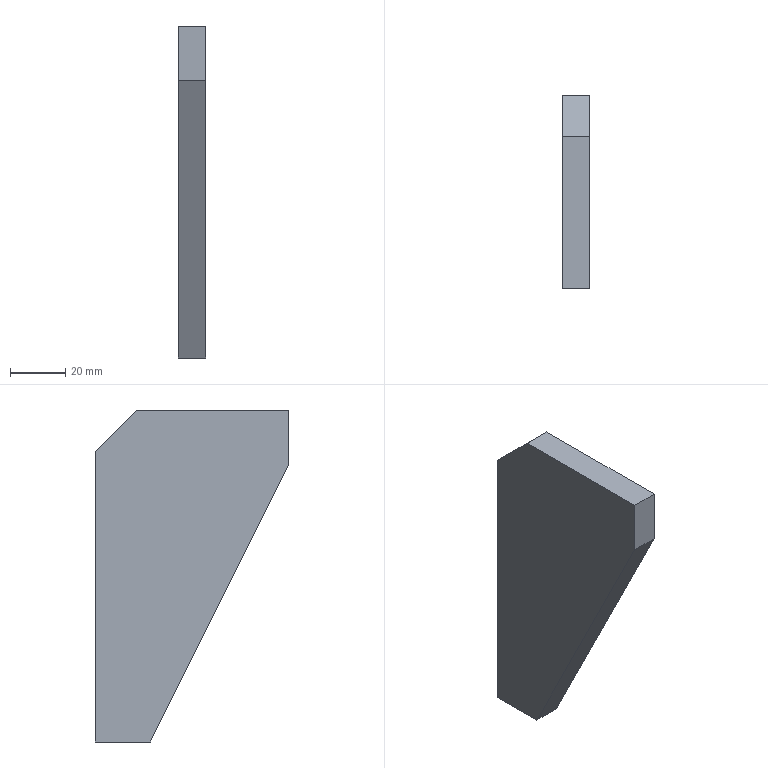Part | STEP file | VD-SYL0380DJ1006_1_4-2_VD-SYL03 | 1 solid | 8 faces | box 10 x 70 x 120 mm | volume 57804 mm3 | plane 8
STEP:
#1=CARTESIAN_POINT('',(0.,0.,-120.));
#2=VERTEX_POINT('',#1);
#3=CARTESIAN_POINT('',(0.,-20.,-120.));
#4=VERTEX_POINT('',#3);
#5=CARTESIAN_POINT('',(0.,0.,-120.));
#6=DIRECTION('',(0.,-1.,0.));
#7=VECTOR('',#6,1000.);
#8=LINE('',#5,#7);
#9=EDGE_CURVE('',#2,#4,#8,.T.);
#10=ORIENTED_EDGE('',*,*,#9,.T.);
#11=CARTESIAN_POINT('',(0.,-70.,-19.716));
#12=VERTEX_POINT('',#11);
#13=CARTESIAN_POINT('',(0.,-20.,-120.));
#14=DIRECTION('',(0.,-0.4462,0.8949));
#15=VECTOR('',#14,1000.);
#16=LINE('',#13,#15);
#17=EDGE_CURVE('',#4,#12,#16,.T.);
#18=ORIENTED_EDGE('',*,*,#17,.T.);
#19=CARTESIAN_POINT('',(0.,-70.,0.));
#20=VERTEX_POINT('',#19);
#21=CARTESIAN_POINT('',(0.,-70.,-19.716));
#22=DIRECTION('',(0.,0.,1.));
#23=VECTOR('',#22,1000.);
#24=LINE('',#21,#23);
#25=EDGE_CURVE('',#12,#20,#24,.T.);
#26=ORIENTED_EDGE('',*,*,#25,.T.);
#27=CARTESIAN_POINT('',(0.,-15.,0.));
#28=VERTEX_POINT('',#27);
#29=CARTESIAN_POINT('',(0.,-70.,0.));
#30=DIRECTION('',(0.,1.,0.));
#31=VECTOR('',#30,1000.);
#32=LINE('',#29,#31);
#33=EDGE_CURVE('',#20,#28,#32,.T.);
#34=ORIENTED_EDGE('',*,*,#33,.T.);
#35=CARTESIAN_POINT('',(0.,0.,-15.));
#36=VERTEX_POINT('',#35);
#37=CARTESIAN_POINT('',(0.,-15.,0.));
#38=DIRECTION('',(0.,0.7071,-0.7071));
#39=VECTOR('',#38,1000.);
#40=LINE('',#37,#39);
#41=EDGE_CURVE('',#28,#36,#40,.T.);
#42=ORIENTED_EDGE('',*,*,#41,.T.);
#43=CARTESIAN_POINT('',(0.,0.,-15.));
#44=DIRECTION('',(0.,0.,-1.));
#45=VECTOR('',#44,1000.);
#46=LINE('',#43,#45);
#47=EDGE_CURVE('',#36,#2,#46,.T.);
#48=ORIENTED_EDGE('',*,*,#47,.T.);
#49=EDGE_LOOP('',(#10,#18,#26,#34,#42,#48));
#50=FACE_OUTER_BOUND('',#49,.T.);
#51=CARTESIAN_POINT('',(0.,0.,0.));
#52=DIRECTION('',(1.,0.,0.));
#53=DIRECTION('',(0.,1.,0.));
#54=AXIS2_PLACEMENT_3D('',#51,#52,#53);
#55=PLANE('',#54);
#56=ADVANCED_FACE('',(#50),#55,.F.);
#57=ORIENTED_EDGE('',*,*,#33,.F.);
#58=CARTESIAN_POINT('',(10.,-70.,0.));
#59=VERTEX_POINT('',#58);
#60=CARTESIAN_POINT('',(0.,-70.,0.));
#61=DIRECTION('',(1.,0.,0.));
#62=VECTOR('',#61,1000.);
#63=LINE('',#60,#62);
#64=EDGE_CURVE('',#20,#59,#63,.T.);
#65=ORIENTED_EDGE('',*,*,#64,.T.);
#66=CARTESIAN_POINT('',(10.,-15.,0.));
#67=VERTEX_POINT('',#66);
#68=CARTESIAN_POINT('',(10.,-15.,0.));
#69=DIRECTION('',(0.,-1.,0.));
#70=VECTOR('',#69,1000.);
#71=LINE('',#68,#70);
#72=EDGE_CURVE('',#67,#59,#71,.T.);
#73=ORIENTED_EDGE('',*,*,#72,.F.);
#74=CARTESIAN_POINT('',(10.,-15.,0.));
#75=DIRECTION('',(-1.,0.,0.));
#76=VECTOR('',#75,1000.);
#77=LINE('',#74,#76);
#78=EDGE_CURVE('',#67,#28,#77,.T.);
#79=ORIENTED_EDGE('',*,*,#78,.T.);
#80=EDGE_LOOP('',(#57,#65,#73,#79));
#81=FACE_OUTER_BOUND('',#80,.T.);
#82=CARTESIAN_POINT('',(0.,-15.,0.));
#83=DIRECTION('',(0.,0.,1.));
#84=DIRECTION('',(1.,0.,0.));
#85=AXIS2_PLACEMENT_3D('',#82,#83,#84);
#86=PLANE('',#85);
#87=ADVANCED_FACE('',(#81),#86,.T.);
#88=ORIENTED_EDGE('',*,*,#25,.F.);
#89=CARTESIAN_POINT('',(10.,-70.,-19.716));
#90=VERTEX_POINT('',#89);
#91=CARTESIAN_POINT('',(0.,-70.,-19.716));
#92=DIRECTION('',(1.,0.,0.));
#93=VECTOR('',#92,1000.);
#94=LINE('',#91,#93);
#95=EDGE_CURVE('',#12,#90,#94,.T.);
#96=ORIENTED_EDGE('',*,*,#95,.T.);
#97=CARTESIAN_POINT('',(10.,-70.,0.));
#98=DIRECTION('',(0.,0.,-1.));
#99=VECTOR('',#98,1000.);
#100=LINE('',#97,#99);
#101=EDGE_CURVE('',#59,#90,#100,.T.);
#102=ORIENTED_EDGE('',*,*,#101,.F.);
#103=ORIENTED_EDGE('',*,*,#64,.F.);
#104=EDGE_LOOP('',(#88,#96,#102,#103));
#105=FACE_OUTER_BOUND('',#104,.T.);
#106=CARTESIAN_POINT('',(0.,-70.,0.));
#107=DIRECTION('',(0.,-1.,0.));
#108=DIRECTION('',(0.,0.,-1.));
#109=AXIS2_PLACEMENT_3D('',#106,#107,#108);
#110=PLANE('',#109);
#111=ADVANCED_FACE('',(#105),#110,.T.);
#112=ORIENTED_EDGE('',*,*,#17,.F.);
#113=CARTESIAN_POINT('',(10.,-20.,-120.));
#114=VERTEX_POINT('',#113);
#115=CARTESIAN_POINT('',(0.,-20.,-120.));
#116=DIRECTION('',(1.,0.,0.));
#117=VECTOR('',#116,1000.);
#118=LINE('',#115,#117);
#119=EDGE_CURVE('',#4,#114,#118,.T.);
#120=ORIENTED_EDGE('',*,*,#119,.T.);
#121=CARTESIAN_POINT('',(10.,-70.,-19.716));
#122=DIRECTION('',(0.,0.4462,-0.8949));
#123=VECTOR('',#122,1000.);
#124=LINE('',#121,#123);
#125=EDGE_CURVE('',#90,#114,#124,.T.);
#126=ORIENTED_EDGE('',*,*,#125,.F.);
#127=ORIENTED_EDGE('',*,*,#95,.F.);
#128=EDGE_LOOP('',(#112,#120,#126,#127));
#129=FACE_OUTER_BOUND('',#128,.T.);
#130=CARTESIAN_POINT('',(0.,-70.,-19.716));
#131=DIRECTION('',(0.,-0.8949,-0.4462));
#132=DIRECTION('',(0.,0.4462,-0.8949));
#133=AXIS2_PLACEMENT_3D('',#130,#131,#132);
#134=PLANE('',#133);
#135=ADVANCED_FACE('',(#129),#134,.T.);
#136=ORIENTED_EDGE('',*,*,#9,.F.);
#137=CARTESIAN_POINT('',(10.,0.,-120.));
#138=VERTEX_POINT('',#137);
#139=CARTESIAN_POINT('',(0.,0.,-120.));
#140=DIRECTION('',(1.,0.,0.));
#141=VECTOR('',#140,1000.);
#142=LINE('',#139,#141);
#143=EDGE_CURVE('',#2,#138,#142,.T.);
#144=ORIENTED_EDGE('',*,*,#143,.T.);
#145=CARTESIAN_POINT('',(10.,-20.,-120.));
#146=DIRECTION('',(0.,1.,0.));
#147=VECTOR('',#146,1000.);
#148=LINE('',#145,#147);
#149=EDGE_CURVE('',#114,#138,#148,.T.);
#150=ORIENTED_EDGE('',*,*,#149,.F.);
#151=ORIENTED_EDGE('',*,*,#119,.F.);
#152=EDGE_LOOP('',(#136,#144,#150,#151));
#153=FACE_OUTER_BOUND('',#152,.T.);
#154=CARTESIAN_POINT('',(0.,-20.,-120.));
#155=DIRECTION('',(0.,0.,-1.));
#156=DIRECTION('',(0.,-1.,0.));
#157=AXIS2_PLACEMENT_3D('',#154,#155,#156);
#158=PLANE('',#157);
#159=ADVANCED_FACE('',(#153),#158,.T.);
#160=ORIENTED_EDGE('',*,*,#47,.F.);
#161=CARTESIAN_POINT('',(10.,0.,-15.));
#162=VERTEX_POINT('',#161);
#163=CARTESIAN_POINT('',(0.,0.,-15.));
#164=DIRECTION('',(1.,0.,0.));
#165=VECTOR('',#164,1000.);
#166=LINE('',#163,#165);
#167=EDGE_CURVE('',#36,#162,#166,.T.);
#168=ORIENTED_EDGE('',*,*,#167,.T.);
#169=CARTESIAN_POINT('',(10.,0.,-120.));
#170=DIRECTION('',(0.,0.,1.));
#171=VECTOR('',#170,1000.);
#172=LINE('',#169,#171);
#173=EDGE_CURVE('',#138,#162,#172,.T.);
#174=ORIENTED_EDGE('',*,*,#173,.F.);
#175=ORIENTED_EDGE('',*,*,#143,.F.);
#176=EDGE_LOOP('',(#160,#168,#174,#175));
#177=FACE_OUTER_BOUND('',#176,.T.);
#178=CARTESIAN_POINT('',(0.,0.,-120.));
#179=DIRECTION('',(0.,1.,0.));
#180=DIRECTION('',(1.,0.,0.));
#181=AXIS2_PLACEMENT_3D('',#178,#179,#180);
#182=PLANE('',#181);
#183=ADVANCED_FACE('',(#177),#182,.T.);
#184=ORIENTED_EDGE('',*,*,#41,.F.);
#185=ORIENTED_EDGE('',*,*,#78,.F.);
#186=CARTESIAN_POINT('',(10.,0.,-15.));
#187=DIRECTION('',(0.,-0.7071,0.7071));
#188=VECTOR('',#187,1000.);
#189=LINE('',#186,#188);
#190=EDGE_CURVE('',#162,#67,#189,.T.);
#191=ORIENTED_EDGE('',*,*,#190,.F.);
#192=ORIENTED_EDGE('',*,*,#167,.F.);
#193=EDGE_LOOP('',(#184,#185,#191,#192));
#194=FACE_OUTER_BOUND('',#193,.T.);
#195=CARTESIAN_POINT('',(0.,0.,-15.));
#196=DIRECTION('',(0.,0.7071,0.7071));
#197=DIRECTION('',(1.,0.,0.));
#198=AXIS2_PLACEMENT_3D('',#195,#196,#197);
#199=PLANE('',#198);
#200=ADVANCED_FACE('',(#194),#199,.T.);
#201=ORIENTED_EDGE('',*,*,#72,.T.);
#202=ORIENTED_EDGE('',*,*,#101,.T.);
#203=ORIENTED_EDGE('',*,*,#125,.T.);
#204=ORIENTED_EDGE('',*,*,#149,.T.);
#205=ORIENTED_EDGE('',*,*,#173,.T.);
#206=ORIENTED_EDGE('',*,*,#190,.T.);
#207=EDGE_LOOP('',(#201,#202,#203,#204,#205,#206));
#208=FACE_OUTER_BOUND('',#207,.T.);
#209=CARTESIAN_POINT('',(10.,0.,0.));
#210=DIRECTION('',(1.,0.,0.));
#211=DIRECTION('',(0.,1.,0.));
#212=AXIS2_PLACEMENT_3D('',#209,#210,#211);
#213=PLANE('',#212);
#214=ADVANCED_FACE('',(#208),#213,.T.);
#215=CLOSED_SHELL('',(#56,#87,#111,#135,#159,#183,#200,#214));
#216=MANIFOLD_SOLID_BREP('',#215);
#217=CARTESIAN_POINT('',(0.,0.,0.));
#218=DIRECTION('',(0.,0.,1.));
#219=DIRECTION('',(1.,0.,0.));
#220=AXIS2_PLACEMENT_3D('',#217,#218,#219);
#221=(LENGTH_UNIT()NAMED_UNIT(*)SI_UNIT(.MILLI.,.METRE.));
#222=UNCERTAINTY_MEASURE_WITH_UNIT(LENGTH_MEASURE(0.00001),#221,'','');
#223=(NAMED_UNIT(*)PLANE_ANGLE_UNIT()SI_UNIT($,.RADIAN.));
#224=(NAMED_UNIT(*)SI_UNIT($,.STERADIAN.)SOLID_ANGLE_UNIT());
#225=(GEOMETRIC_REPRESENTATION_CONTEXT(3)GLOBAL_UNCERTAINTY_ASSIGNED_CONTEXT((#222))GLOBAL_UNIT_ASSIGNED_CONTEXT((#221,#223,#224))REPRESENTATION_CONTEXT('',''));
#226=ADVANCED_BREP_SHAPE_REPRESENTATION('',(#216,#220),#225);